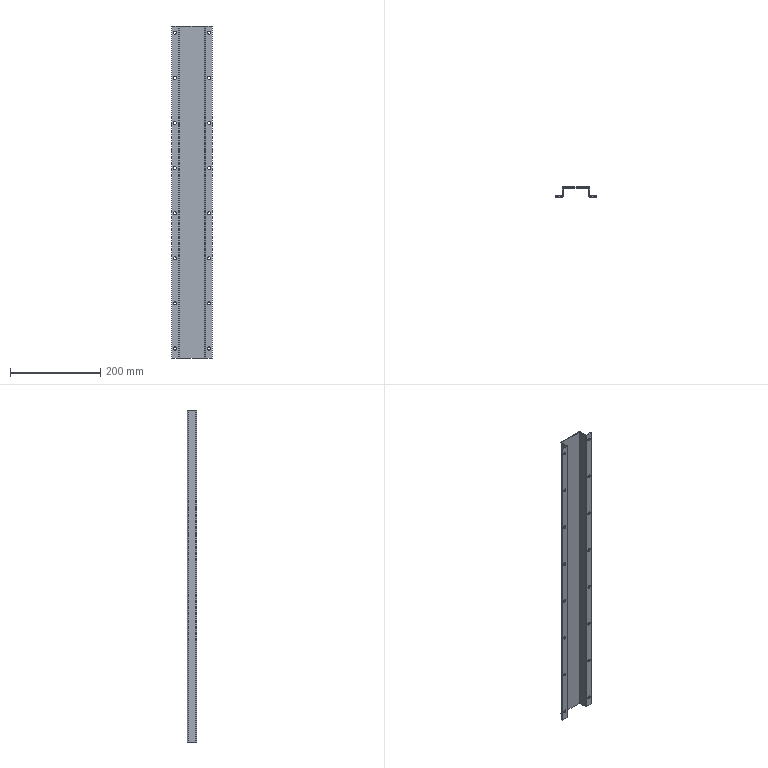Part | STEP file | Center Shaft Plate Rib | 1 solid | 54 faces | box 90 x 22 x 736 mm | volume 186338 mm3 | cylinder 40 | plane 14 | commonest cylinder face diameters 7 x32 1 x4 5 x4